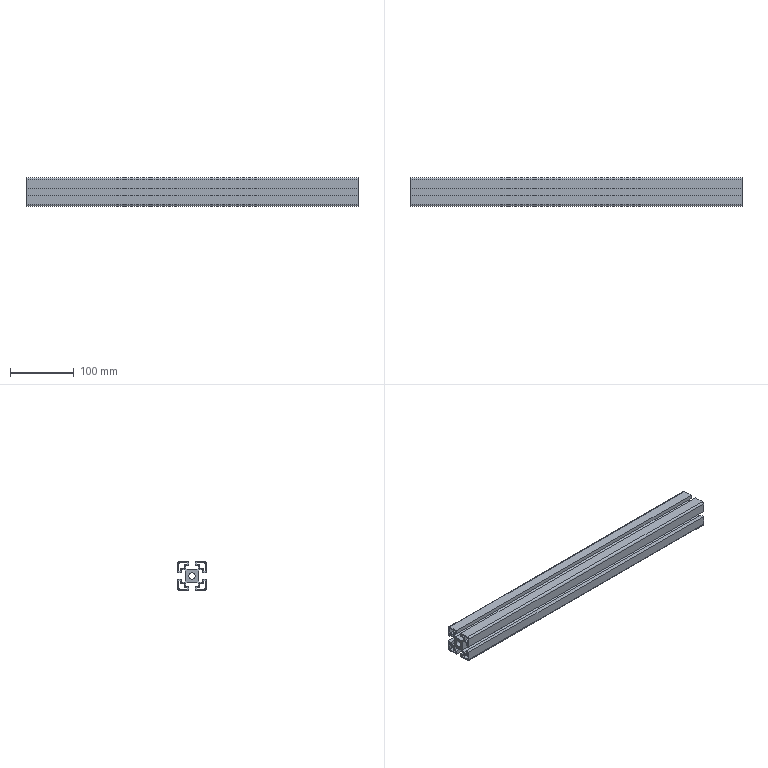Part | STEP file | 1_10 | 1 solid | 87 faces | box 520 x 45 x 45 mm | volume 425226 mm3 | plane 78 | cylinder 9 | commonest cylinder face diameters 2 x4 6 x4 10 x1